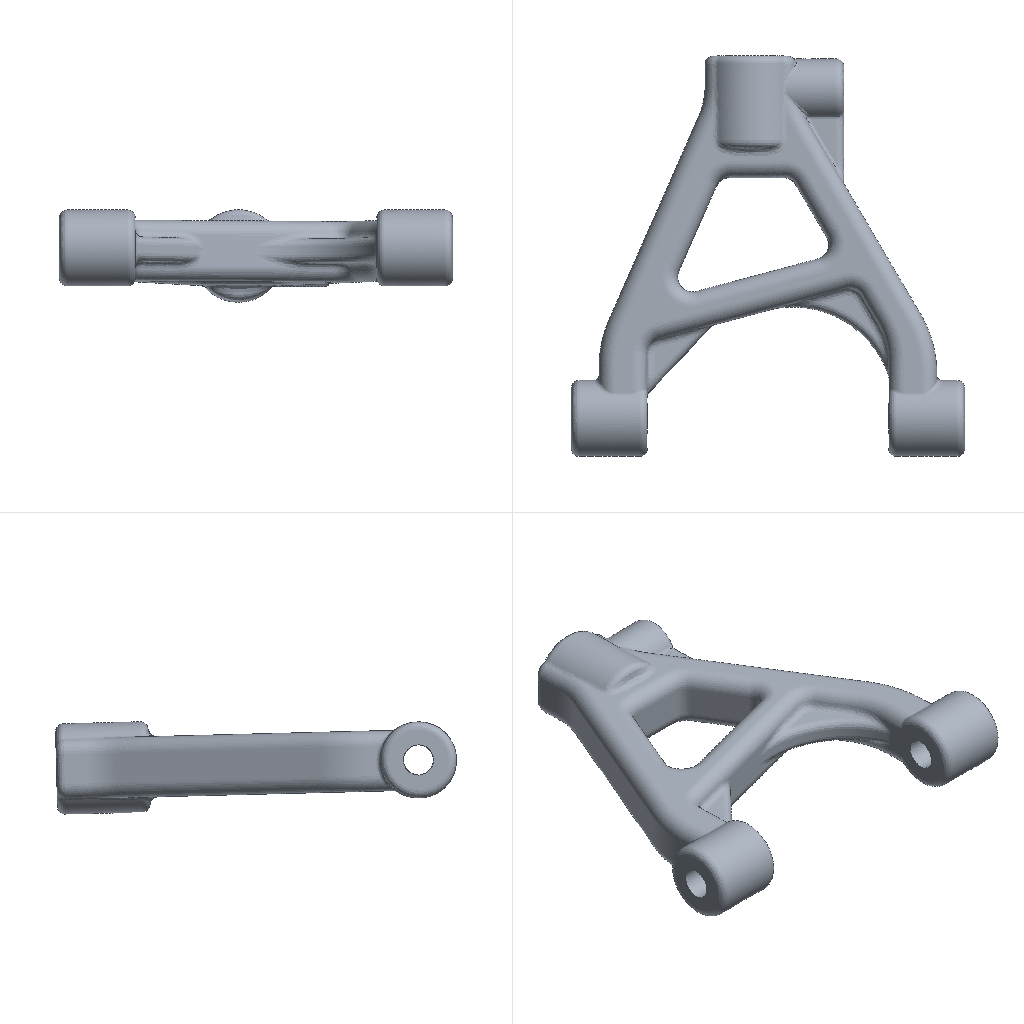Simulation study | ansys workbench
Set-up summary:
category,name,step,type,value,unit,region
solver,ansys_mapdl
solver,version,,,21.1
units,MPA,,stated
analysis,deck,,static,static
load_step,requested,,,1
analysis,nlgeom,,,False
mesh,nodes,,,931882
mesh,elements,,,640923
element_type,ANSYS 187 (type 1),,solid,640161
element_type,ANSYS 154 (type 2),,surface,762
load,load commands in deck,,count,3
bc,support commands in deck,,count,1
named_set,_FIXEDSU,,component
material,1,,in results
check,setup vs results,,match,762 surface effect element(s) are not in the reader's mesh and were not compared
Ansys APDL input file, long lists of numbers shortened:
/batch
/config,noeldb,1     ! force off writing results to database
*get,_wallstrt,active,,time,wall
! ANSYS input file written by Workbench version 2021 R1
! File used for geometry attach: D:\仿真\支臂分析优化2025.05.07\模型\下支臂2.0.STEP
/title,_____--5000N____ (D5)
! ****** Begin Custom Load Command Snippet ******
/COM, ACT Extensions:
/COM,     LSDYNA, 2021.1
/COM,
! ****** End   Custom Load Command Snippet ******
*DIM,_wb_ProjectScratch_dir,string,248
_wb_ProjectScratch_dir(1) = 'D:\仿真\支臂分析优化2025.05.07\_ProjectScratch\ScrD1CD\'
*DIM,_wb_SolverFiles_dir,string,248
_wb_SolverFiles_dir(1) = 'D:\仿真\支臂分析优化2025.05.07\下支臂仿真_files\dp0\SYS-4\MECH\'
*DIM,_wb_userfiles_dir,string,248
_wb_userfiles_dir(1) = 'D:\仿真\支臂分析优化2025.05.07\下支臂仿真_files\user_files\'
/com,--- Data in consistent NMM units. See Solving Units in the help system for more information.
/units,MPA
/nopr
/wb,file,start              !  signify a WB generated input file
/prep7
! Turn off shape checking because checks already performed inside WB mesher.
! See help system for more information.
SHPP,OFF,,NOWARN
/nolist
etcon,set             ! allow ANSYS to choose best KEYOP's for 180x elements, resets any applicable keyopt to MAPDL defaults
/com,*********** Nodes for the whole assembly ***********
nblock,3,,1025070
(1i9,3e20.9e3)
        1     1.723915954E+02    -8.593183532E+01    -3.788723736E+01
! (931881 more lines like these left out)
-1
/wb,elem,start            !  set before creation of elements
/com,*********** Elements for Body 1 "___2-FreeParts|____3" ***********
et,1,187
eblock,19,solid,,640161
(19i9)
        1        1        1        1        0        0        0        0       10        0        1    62359   126301   126559   126555   619691   931862   619693   619692
! (1280321 more lines like these left out)
-1
/wb,elem,end               !  done creating elements
/com,*********** Send User Defined Coordinate System(s) ***********
csys,0
toffst,273.15,  ! Temperature offset from absolute zero
/com,*********** Set Reference Temperature ***********
tref,22.
/wb,mat,start              !  starting to send materials
/com,*********** Send Materials ***********
Temperature = 'TEMP' ! Temperature
MP,DENS,1,7.85e-09,	! tonne mm^-3
MP,ALPX,1,1.2e-05,	! C^-1
MP,C,1,434000000,	! mm^2 s^-2 C^-1
MP,KXX,1,60.5,	! tonne mm s^-3 C^-1
MP,RSVX,1,0.00017,	! ohm mm
MP,EX,1,200000,	! tonne s^-2 mm^-1
MP,NUXY,1,0.3,
MP,MURX,1,10000,
/wb,mat,end                !  done sending materials
!************************* Model Summary ********************
!___2-FreeParts|____3,	结构钢,	matid,	1
!************************* End Model Summary ********************
! get the diagonal of the bounding box. Needed later for other things
*get,_xmin,node,,mnloc,x
*get,_ymin,node,,mnloc,y
*get,_zmin,node,,mnloc,z
*get,_xmax,node,,mxloc,x
*get,_ymax,node,,mxloc,y
*get,_zmax,node,,mxloc,z
_ASMDIAG=(_xmax-_xmin)*(_xmax-_xmin)+(_ymax-_ymin)*(_ymax-_ymin)+(_zmax-_zmin)*(_zmax-_zmin)
_ASMDIAG=SQRT(_ASMDIAG)
/wb,contact,start          !  starting to send contact
/wb,contact,end            !  done creating contacts
/golist
/wb,load,start             !  starting to send loads
/com,*********** Fixed Supports ***********
CMBLOCK,_FIXEDSU,NODE,     9156
(8i10)
       390       391       392       393       394       395       396       397
! (1144 more lines like these left out)
cmsel,s,_FIXEDSU
d,all,all
nsel,all
/com,*********** Define Force Using Surface Effect Elements ***********
local,12,0,0.,0.,0.,0.,0.,0.
csys,0
et,2,154
eblock,10,,,762
(15i9)
   717364        2        2        2       12    35148    35216    35329    35329   363476   364114    35329   363480
! (761 more lines like these left out)
-1
esel,s,type,,2
keyop,2,2,1                ! Apply load in local coordinate system
keyop,2,7,1                ! Use original area so load is constant in large deformation
esel,all
*DIM,_loadvari30z,TABLE,2,1,1,TIME,
! Time values
_loadvari30z(1,0,1) = 0.
_loadvari30z(2,0,1) = 1.
! Load values
_loadvari30z(1,1,1) = 3.505
_loadvari30z(2,1,1) = 3.505
/gst,on,on
fini
*get,_numnode,node,0,count
*get,_numelem,elem,0,count
*get, _MAXELEMNUM, elem, 0, NUM, MAX
*get, _MAXNODENUM, node, 0, NUM, MAX
*get, _MAXELEMTYPE, etyp, 0, NUM, MAX
*get, _MAXREALCONST, real, 0, NUM, MAX
/go
/wb,load,end               !  done creating loads
/com,--- Number of total nodes = %_numnode%
/com,--- Number of contact elements = 762
/com,--- Number of spring elements = 0
/com,--- Number of bearing elements = 0
/com,--- Number of solid elements = 640161
/com,--- Number of condensed parts = 0
/com,--- Number of total elements = %_numelem%
*get,_wallbsol,active,,time,wall
/com,****************************************************************************
/com,*************************    SOLUTION       ********************************
/com,****************************************************************************
/solu
antype,0                   ! static analysis
_thickRatio=  1     ! Ratio of thick parts in the model
eqsl,pcg,1e-8,,,,,,1
cntr,print,1               ! print out contact info and also make no initial contact an error
dmpoption,emat,no             ! Don't combine emat file for DANSYS
dmpoption,esav,no             ! Don't combine esav file for DANSYS
nldiag,cont,iter           ! print out contact info each equilibrium iteration
rescontrol,,none                 ! Do not keep any restart files
/com,****************************************************
/com,******************* SOLVE FOR LS 1 OF 1 ****************
esel,s,type,,2
nsle
sfe,all,1,pres,1,0.
sfe,all,2,pres,1,0.
sfe,all,3,pres,1,%_loadvari30z%
nsel,all
esel,all
/nopr
/gopr
/nolist
nsub,1,1,1
time,1.
outres,erase
outres,all,none
outres,nsol,all,
outres,rsol,all
outres,eangl,all
outres,etmp,all
outres,veng,all
outres,strs,all,
outres,epel,all,
outres,eppl,all,
outres,cont,all,
! *********** WB SOLVE COMMAND ***********
! check interactive state
*get,ANSINTER_,active,,int
*if,ANSINTER_,ne,0,then
/eof
*endif
solve
/com *************** Write FE CONNECTORS *********
CEWRITE,file,ce,,INTE
/com,****************************************************
/com,*************** FINISHED SOLVE FOR LS 1 *************
*get,_wallasol,active,,time,wall
/nopr
*get,_numnode,node,0,count
*get,_numelem,elem,0,count
*get, _MAXELEMNUM, elem, 0, NUM, MAX
*get, _MAXNODENUM, node, 0, NUM, MAX,,,INTERNAL
*get, _MAXELEMTYPE, etyp, 0, NUM, MAX
*get, _MAXREALCONST, real, 0, NUM, MAX
/gopr
*get,_PCGITER,active,,solu,cgiter
/post1
xmlo,ENCODING,ISO-8859-1
xmlo,parm
/xml,parm,xml
fini
/gopr
*get,_walldone,active,,time,wall
_preptime=(_wallbsol-_wallstrt)*3600
_solvtime=(_wallasol-_wallbsol)*3600
_posttime=(_walldone-_wallasol)*3600
_totaltim=(_walldone-_wallstrt)*3600
*get,_dlbratio,active,0,solu,dlbr
*get,_combtime,active,0,solu,comb
/com,--- Total number of nodes = %_numnode%
/com,--- Total number of elements = %_numelem%
/com,--- Element load balance ratio = %_dlbratio%
/com,--- Time to combine distributed files = %_combtime%
/wb,file,end               ! done with WB generated input
Results summary:
result,analysis,,,static
result,last_loadstep,,,1
result,primary field,,,displacement
result,reaction total,1,FX,4.4e-05,N
result,reaction total,1,FY,1.1e-05,N
result,reaction total,1,FZ,-12500,N
result,mass,,,0.02913,"NMM: mm, ton, N, s, mV, mA, degC"